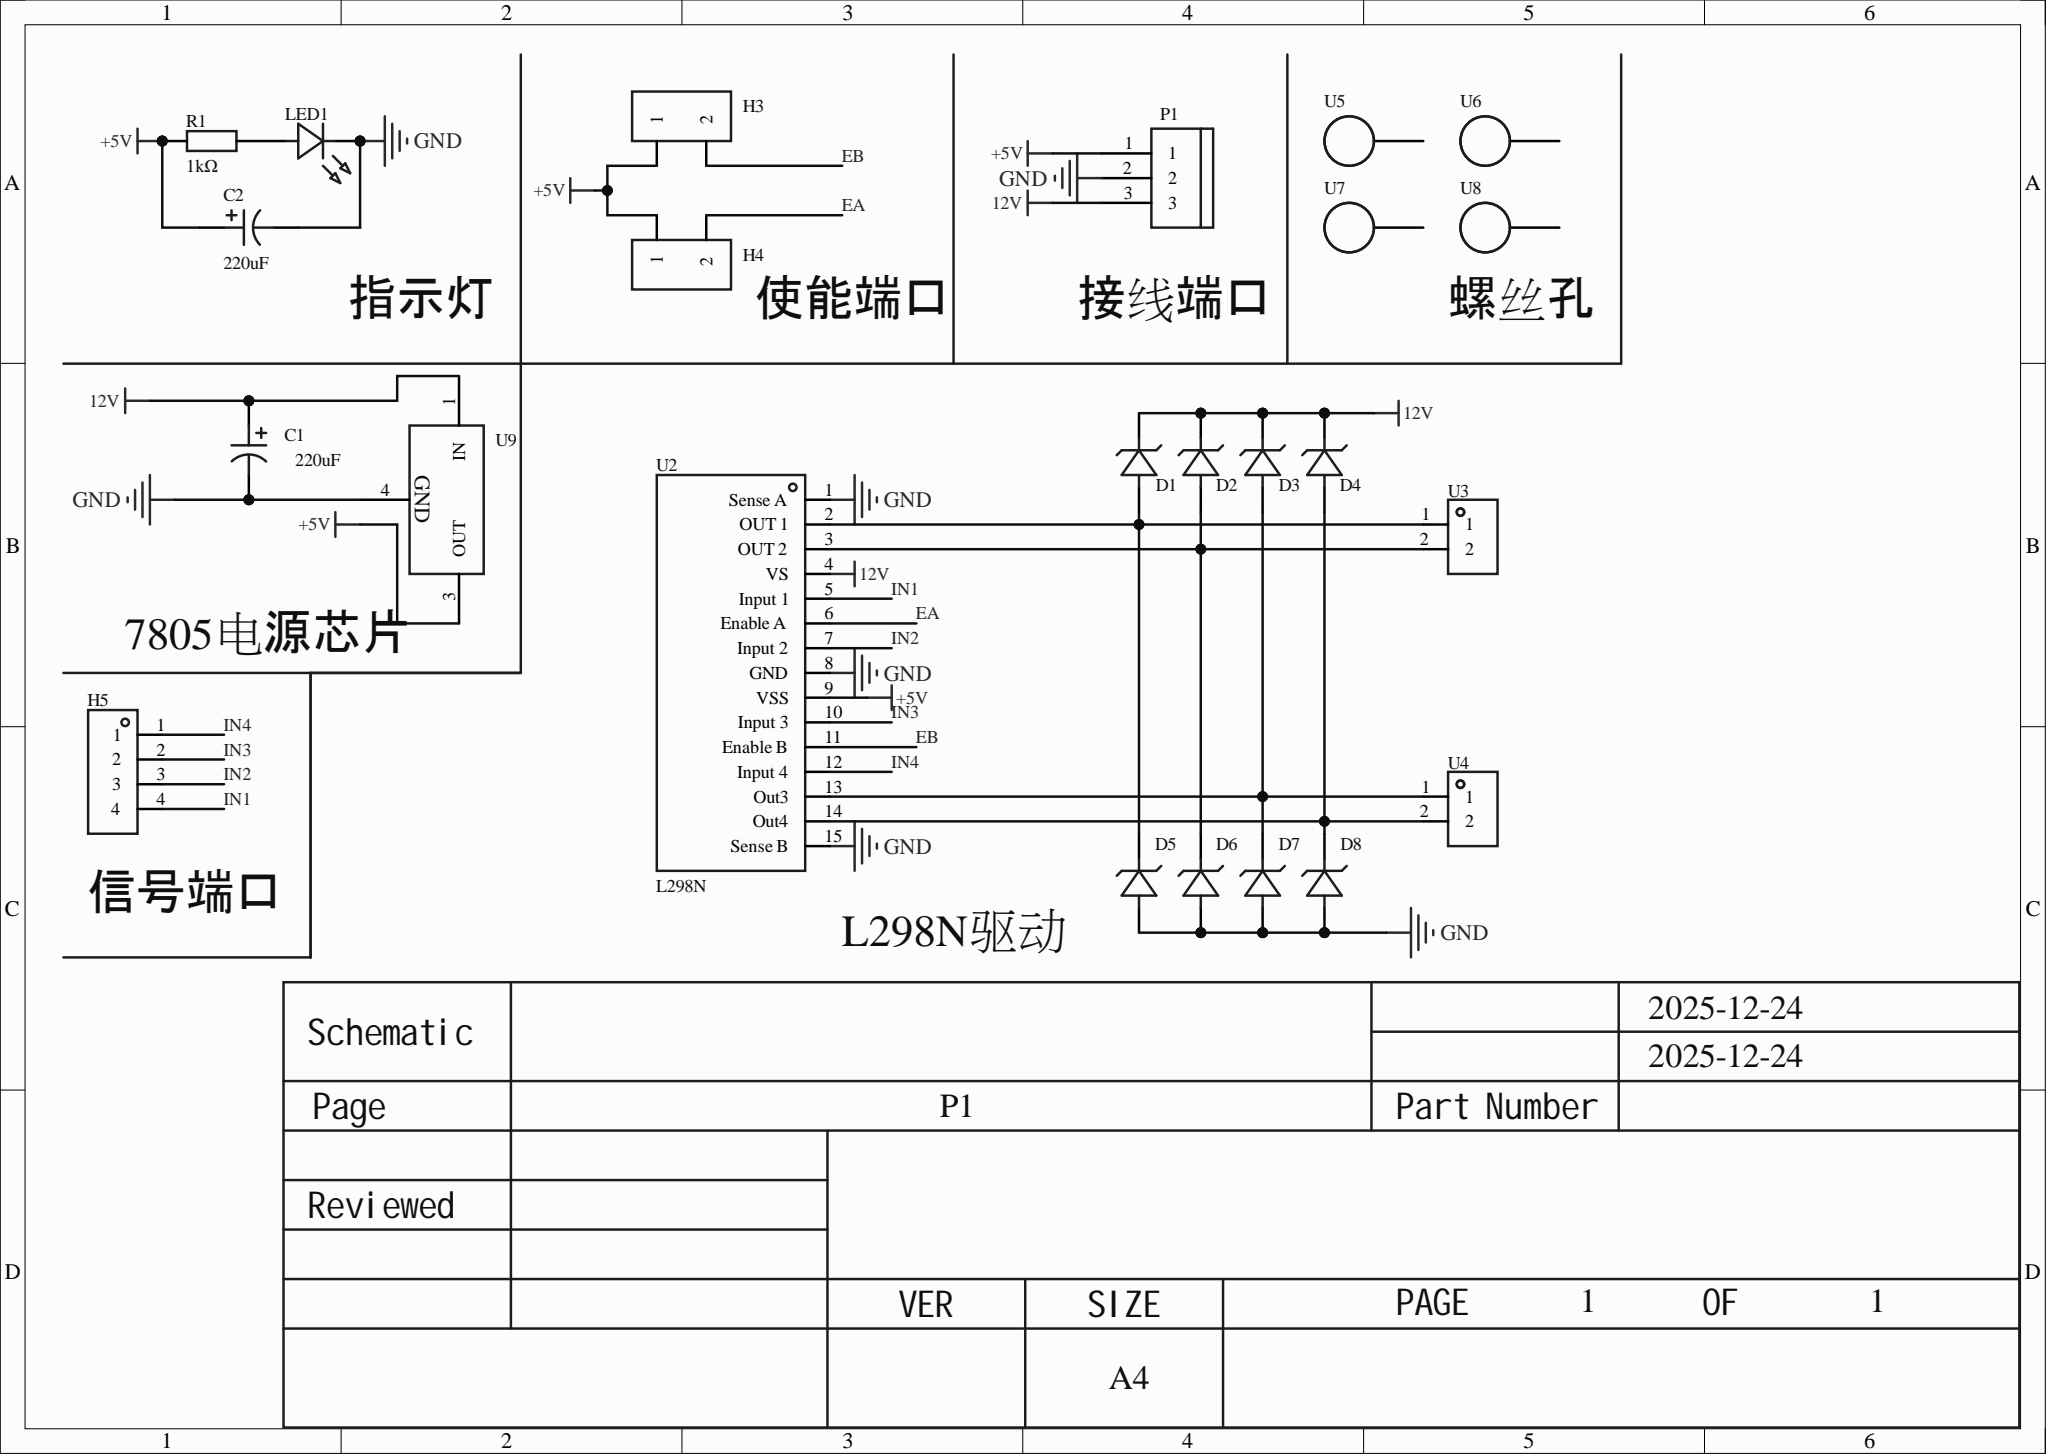Circuit board | Altium Designer | 24 parts | 14 nets
Bill of materials:
Comment,Description,Designator,Footprint,LibRef,Quantity
"","容值:220uF;精度:±20%;额定电压:35V;电容体直径:-;电容体长度:-;纹波电流:-;等效串联电阻:-;工作寿命:-;工作温度:-;","C1, C2","CAP-SMD_BD8.0-L8.3-W8.3-LS9.3-FD","EMK1VM221FB0D00R","2"
"","二极管配置:独立式;直流反向耐压(Vr):1kV;平均整流电流(Io):1A;正向压降(Vf):1.1V@1A;反向电流(Ir):10A@1kV;","D1, D2, D3, D4, D5, D6, D7, D8","SOD-123FL_L2.7-W1.8-LS3.8-RD","1N4007","8"
"","间距:2.54mm;总PIN位数:2;排数:1;插针结构:-;行距:-;安装类型:直插;圆针/方针:-;额定电流:-;额定电压:-;配合针长度:-;塑高:-;触头材质:黄铜;触头镀层:-;颜色:绿色;","H3, H4","HDR-TH_2P-P2.54-V-M-1","826629-2","2"
"826629-4","排数:单排;总PIN位数:4;间距:2.54mm;插针结构:1x4P;行距:-;安装类型:直插;圆针/方针:-;额定电流:-;额定电压:-;配合针长度:6.7mm;塑高:2.8mm;端接针长度:3.2mm;触头材质:-;工作温度范围:-;颜色:绿色;","H5","HDR-TH_4P-P2.54-V-M-1","826629-4","1"
"","发光颜色:蓝灯;二极管配置:-;透镜颜色:-;主波长:-;峰值波长:-;色温:-;光通量(25时):-;测试电流:20mA;正向电压(VF):-;发光强度:-;功率:70mW;发光角度:140°;安装方式:正贴;工作温度:-40~+85;","LED1","LED0805-RD_BLUE","RF-BGB170TS-CB-E0","1"
"","间距:5.08mm;排数:1;每排PIN数:3;安装方式:直针;额定电流:18A;额定电压:250V;线规 - AWG:14~30;线规 - mm?:2.5;工作温度范围:-40~+105;颜色:绿色;","P1","CONN-TH_3P-P5.00_WJ500V-5.08-3P","WJ500V-5.08-3P","1"
"","","R1","R0805","RS-05K102JT","1"
"L298N","电源电压:4.5V~7V;特性:过流保护(OCP)；过热保护(OPT);","U2","MULTIWATT-15_L19.6-W5.0-P1.27-L","L298N_C19922","1"
"","","U3, U4","CONN-TH_DB302-5.0-2P","DB302-5.0-2P-GN-S","2"
"","螺柱类型:单通螺柱;公称直径:M3;螺距:-;长度:11mm;执行标准:-;强度等级:-;材料:-;表面处理:-;","U5, U6, U7, U8","SMD_BD4.2-L4.7-W4.7-D3.0","铜柱M3*5+6","4"
"L78M05ABDT-TR","L78M Series 500 mA 5 V Three Terminal Positive Voltage LDO Regulator - TO-252","U9","TO-252-2_L6.5-W6.1-P4.58-LS10.0-TL","L78M05ABDT-TR","1"
Netlist (Protel format):
[
C1
CAP-SMD_BD8.0-L8.3-W8.3-LS9.3-FD




]
[
C2
CAP-SMD_BD8.0-L8.3-W8.3-LS9.3-FD




]
[
D1
SOD-123FL_L2.7-W1.8-LS3.8-RD




]
[
D2
SOD-123FL_L2.7-W1.8-LS3.8-RD




]
[
D3
SOD-123FL_L2.7-W1.8-LS3.8-RD




]
[
D4
SOD-123FL_L2.7-W1.8-LS3.8-RD




]
[
D5
SOD-123FL_L2.7-W1.8-LS3.8-RD




]
[
D6
SOD-123FL_L2.7-W1.8-LS3.8-RD




]
[
D7
SOD-123FL_L2.7-W1.8-LS3.8-RD




]
[
D8
SOD-123FL_L2.7-W1.8-LS3.8-RD




]
[
H3
HDR-TH_2P-P2.54-V-M-1




]
[
H4
HDR-TH_2P-P2.54-V-M-1




]
[
H5
HDR-TH_4P-P2.54-V-M-1
826629-4



]
[
LED1
LED0805-RD_BLUE




]
[
P1
CONN-TH_3P-P5.00_WJ500V-5.08-3P




]
[
R1
R0805




]
[
U2
MULTIWATT-15_L19.6-W5.0-P1.27-L
L298N



]
[
U3
CONN-TH_DB302-5.0-2P




]
[
U4
CONN-TH_DB302-5.0-2P




]
[
U5
SMD_BD4.2-L4.7-W4.7-D3.0




]
[
U6
SMD_BD4.2-L4.7-W4.7-D3.0




]
[
U7
SMD_BD4.2-L4.7-W4.7-D3.0




]
[
U8
SMD_BD4.2-L4.7-W4.7-D3.0




]
[
U9
TO-252-2_L6.5-W6.1-P4.58-LS10.0-TL
L78M05ABDT-TR



]
(
NetLED1_2
LED1-2
R1-1
)
(
NetD4_2
D4-2
D8-1
U2-14
U4-2
)
(
NetD3_2
D3-2
D7-1
U2-13
U4-1
)
(
NetD2_2
D2-2
D6-1
U2-3
U3-2
)
(
NetD1_2
D1-2
D5-1
U2-2
U3-1
)
(
IN4
H5-1
U2-12
)
(
IN3
H5-2
U2-10
)
(
IN2
H5-3
U2-7
)
(
IN1
H5-4
U2-5
)
(
GND
C1-2
C2-2
D5-2
D6-2
D7-2
D8-2
LED1-1
P1-2
U2-1
U2-8
U2-15
U9-4
)
(
EB
H3-2
U2-11
)
(
EA
H4-2
U2-6
)
(
+5V
C2-1
H3-1
H4-1
P1-1
R1-2
U2-9
U9-3
)
(
12V
C1-1
D1-1
D2-1
D3-1
D4-1
P1-3
U2-4
U9-1
)